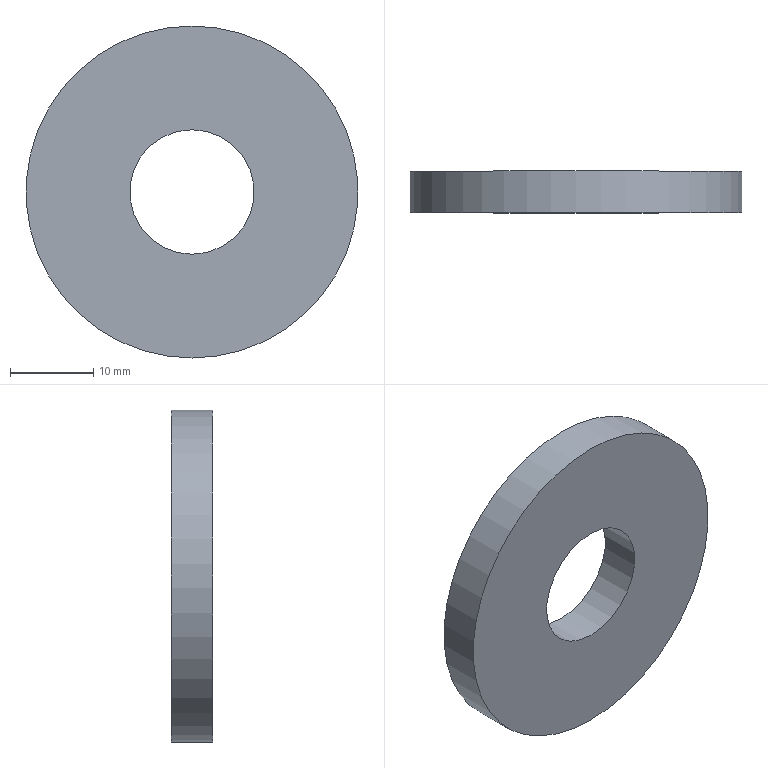Part | STEP file | HL4GZ-1.862.102 flat washer | 1 solid | 4 faces | box 40 x 5 x 40 mm | volume 5400 mm3 | plane 2 | cylinder 2 | commonest cylinder face diameters 15 x1 40 x1
STEP:
#1=CARTESIAN_POINT('',(0.,0.,0.));
#2=DIRECTION('',(0.,0.,1.));
#3=DIRECTION('',(1.,0.,0.));
#4=AXIS2_PLACEMENT_3D('',#1,#2,#3);
#5=CARTESIAN_POINT('',(1892.35,-249.5,-221.665));
#6=VERTEX_POINT('',#5);
#7=CARTESIAN_POINT('',(1885.318,-249.5,-219.057));
#8=DIRECTION('',(0.,1.,0.));
#9=DIRECTION('',(-0.9376,0.,0.3477));
#10=AXIS2_PLACEMENT_3D('',#7,#8,#9);
#11=CIRCLE('',#10,7.5);
#12=CARTESIAN_POINT('',(1885.318,-249.5,-219.057));
#13=DIRECTION('',(0.,-1.,0.));
#14=DIRECTION('',(-0.3477,0.,-0.9376));
#15=AXIS2_PLACEMENT_3D('',#12,#13,#14);
#16=PLANE('',#15);
#17=CARTESIAN_POINT('',(0.,-7.5));
#18=CARTESIAN_POINT('',(-12.99,-7.5));
#19=CARTESIAN_POINT('',(-6.495,3.75));
#20=CARTESIAN_POINT('',(0.,15.));
#21=CARTESIAN_POINT('',(6.495,3.75));
#22=CARTESIAN_POINT('',(12.99,-7.5));
#23=CARTESIAN_POINT('',(0.,-7.5));
#24=(BOUNDED_CURVE()B_SPLINE_CURVE(2,(#17,#18,#19,#20,#21,#22,#23),.UNSPECIFIED.,.T.,.F.)B_SPLINE_CURVE_WITH_KNOTS((1,2,2,2,2,1),(-2.094,0.,2.094,4.189,6.283,8.378),.UNSPECIFIED.)CURVE()GEOMETRIC_REPRESENTATION_ITEM()RATIONAL_B_SPLINE_CURVE((1.,0.5,1.,0.5,1.,0.5,1.))REPRESENTATION_ITEM(''));
#25=(GEOMETRIC_REPRESENTATION_CONTEXT(2)PARAMETRIC_REPRESENTATION_CONTEXT()REPRESENTATION_CONTEXT('',''));
#26=DEFINITIONAL_REPRESENTATION('',(#24),#25);
#27=PCURVE('',#16,#26);
#28=CARTESIAN_POINT('',(1885.318,-247.5,-219.057));
#29=DIRECTION('',(0.,1.,0.));
#30=DIRECTION('',(-0.9376,0.,0.3477));
#31=AXIS2_PLACEMENT_3D('',#28,#29,#30);
#32=CYLINDRICAL_SURFACE('',#31,7.5);
#33=CARTESIAN_POINT('',(0.,-2.));
#34=DIRECTION('',(1.,0.));
#35=VECTOR('',#34,1.);
#36=LINE('',#33,#35);
#37=(GEOMETRIC_REPRESENTATION_CONTEXT(2)PARAMETRIC_REPRESENTATION_CONTEXT()REPRESENTATION_CONTEXT('',''));
#38=DEFINITIONAL_REPRESENTATION('',(#36),#37);
#39=PCURVE('',#32,#38);
#40=SURFACE_CURVE('',#11,(#27,#39),.PCURVE_S1.);
#41=EDGE_CURVE('',#6,#6,#40,.T.);
#42=ORIENTED_EDGE('',*,*,#41,.T.);
#43=EDGE_LOOP('',(#42));
#44=FACE_BOUND('',#43,.T.);
#45=CARTESIAN_POINT('',(1885.318,-249.5,-239.057));
#46=VERTEX_POINT('',#45);
#47=CARTESIAN_POINT('',(1885.318,-249.5,-219.057));
#48=DIRECTION('',(0.,-1.,0.));
#49=DIRECTION('',(0.,0.,-1.));
#50=AXIS2_PLACEMENT_3D('',#47,#48,#49);
#51=CIRCLE('',#50,20.);
#52=CARTESIAN_POINT('',(0.,0.));
#53=DIRECTION('',(0.9376,0.3477));
#54=AXIS2_PLACEMENT_2D('',#52,#53);
#55=CIRCLE('',#54,20.);
#56=(GEOMETRIC_REPRESENTATION_CONTEXT(2)PARAMETRIC_REPRESENTATION_CONTEXT()REPRESENTATION_CONTEXT('',''));
#57=DEFINITIONAL_REPRESENTATION('',(#55),#56);
#58=PCURVE('',#16,#57);
#59=CARTESIAN_POINT('',(1885.318,-247.5,-219.057));
#60=DIRECTION('',(0.,1.,0.));
#61=DIRECTION('',(-0.9376,0.,0.3477));
#62=AXIS2_PLACEMENT_3D('',#59,#60,#61);
#63=CYLINDRICAL_SURFACE('',#62,20.);
#64=CARTESIAN_POINT('',(10.64,-2.));
#65=DIRECTION('',(-1.,0.));
#66=VECTOR('',#65,1.);
#67=LINE('',#64,#66);
#68=(GEOMETRIC_REPRESENTATION_CONTEXT(2)PARAMETRIC_REPRESENTATION_CONTEXT()REPRESENTATION_CONTEXT('',''));
#69=DEFINITIONAL_REPRESENTATION('',(#67),#68);
#70=PCURVE('',#63,#69);
#71=SURFACE_CURVE('',#51,(#58,#70),.PCURVE_S1.);
#72=EDGE_CURVE('',#46,#46,#71,.T.);
#73=ORIENTED_EDGE('',*,*,#72,.T.);
#74=EDGE_LOOP('',(#73));
#75=FACE_BOUND('',#74,.T.);
#76=ADVANCED_FACE('',(#44,#75),#16,.T.);
#77=CARTESIAN_POINT('',(1892.35,-244.5,-221.665));
#78=VERTEX_POINT('',#77);
#79=CARTESIAN_POINT('',(1885.318,-244.5,-219.057));
#80=DIRECTION('',(0.,-1.,0.));
#81=DIRECTION('',(-0.9376,0.,0.3477));
#82=AXIS2_PLACEMENT_3D('',#79,#80,#81);
#83=CIRCLE('',#82,7.5);
#84=CARTESIAN_POINT('',(1885.318,-244.5,-219.057));
#85=DIRECTION('',(0.,-1.,0.));
#86=DIRECTION('',(-0.3477,0.,-0.9376));
#87=AXIS2_PLACEMENT_3D('',#84,#85,#86);
#88=PLANE('',#87);
#89=CARTESIAN_POINT('',(0.,0.));
#90=DIRECTION('',(0.,-1.));
#91=AXIS2_PLACEMENT_2D('',#89,#90);
#92=CIRCLE('',#91,7.5);
#93=(GEOMETRIC_REPRESENTATION_CONTEXT(2)PARAMETRIC_REPRESENTATION_CONTEXT()REPRESENTATION_CONTEXT('',''));
#94=DEFINITIONAL_REPRESENTATION('',(#92),#93);
#95=PCURVE('',#88,#94);
#96=CARTESIAN_POINT('',(12.566,3.));
#97=DIRECTION('',(-1.,0.));
#98=VECTOR('',#97,1.);
#99=LINE('',#96,#98);
#100=(GEOMETRIC_REPRESENTATION_CONTEXT(2)PARAMETRIC_REPRESENTATION_CONTEXT()REPRESENTATION_CONTEXT('',''));
#101=DEFINITIONAL_REPRESENTATION('',(#99),#100);
#102=PCURVE('',#32,#101);
#103=SURFACE_CURVE('',#83,(#95,#102),.PCURVE_S1.);
#104=EDGE_CURVE('',#78,#78,#103,.T.);
#105=ORIENTED_EDGE('',*,*,#104,.T.);
#106=EDGE_LOOP('',(#105));
#107=FACE_BOUND('',#106,.T.);
#108=CARTESIAN_POINT('',(1885.318,-244.5,-239.057));
#109=VERTEX_POINT('',#108);
#110=CARTESIAN_POINT('',(1885.318,-244.5,-219.057));
#111=DIRECTION('',(0.,-1.,0.));
#112=DIRECTION('',(0.,0.,-1.));
#113=AXIS2_PLACEMENT_3D('',#110,#111,#112);
#114=CIRCLE('',#113,20.);
#115=CARTESIAN_POINT('',(0.,0.));
#116=DIRECTION('',(0.9376,0.3477));
#117=AXIS2_PLACEMENT_2D('',#115,#116);
#118=CIRCLE('',#117,20.);
#119=(GEOMETRIC_REPRESENTATION_CONTEXT(2)PARAMETRIC_REPRESENTATION_CONTEXT()REPRESENTATION_CONTEXT('',''));
#120=DEFINITIONAL_REPRESENTATION('',(#118),#119);
#121=PCURVE('',#88,#120);
#122=CARTESIAN_POINT('',(10.64,3.));
#123=DIRECTION('',(-1.,0.));
#124=VECTOR('',#123,1.);
#125=LINE('',#122,#124);
#126=(GEOMETRIC_REPRESENTATION_CONTEXT(2)PARAMETRIC_REPRESENTATION_CONTEXT()REPRESENTATION_CONTEXT('',''));
#127=DEFINITIONAL_REPRESENTATION('',(#125),#126);
#128=PCURVE('',#63,#127);
#129=SURFACE_CURVE('',#114,(#121,#128),.PCURVE_S1.);
#130=EDGE_CURVE('',#109,#109,#129,.T.);
#131=ORIENTED_EDGE('',*,*,#130,.F.);
#132=EDGE_LOOP('',(#131));
#133=FACE_BOUND('',#132,.T.);
#134=ADVANCED_FACE('',(#107,#133),#88,.F.);
#135=ORIENTED_EDGE('',*,*,#72,.F.);
#136=CARTESIAN_POINT('',(1885.318,-249.5,-239.057));
#137=CARTESIAN_POINT('',(1885.318,-244.5,-239.057));
#138=B_SPLINE_CURVE_WITH_KNOTS('',1,(#136,#137),.UNSPECIFIED.,.F.,.F.,(2,2),(-2.,3.),.PIECEWISE_BEZIER_KNOTS.);
#139=CARTESIAN_POINT('',(10.64,0.));
#140=DIRECTION('',(0.,1.));
#141=VECTOR('',#140,1.);
#142=LINE('',#139,#141);
#143=(GEOMETRIC_REPRESENTATION_CONTEXT(2)PARAMETRIC_REPRESENTATION_CONTEXT()REPRESENTATION_CONTEXT('',''));
#144=DEFINITIONAL_REPRESENTATION('',(#142),#143);
#145=PCURVE('',#63,#144);
#146=CARTESIAN_POINT('',(4.357,0.));
#147=DIRECTION('',(0.,1.));
#148=VECTOR('',#147,1.);
#149=LINE('',#146,#148);
#150=(GEOMETRIC_REPRESENTATION_CONTEXT(2)PARAMETRIC_REPRESENTATION_CONTEXT()REPRESENTATION_CONTEXT('',''));
#151=DEFINITIONAL_REPRESENTATION('',(#149),#150);
#152=PCURVE('',#63,#151);
#153=SEAM_CURVE('',#138,(#145,#152),.PCURVE_S1.);
#154=EDGE_CURVE('',#46,#109,#153,.T.);
#155=ORIENTED_EDGE('',*,*,#154,.T.);
#156=ORIENTED_EDGE('',*,*,#130,.T.);
#157=ORIENTED_EDGE('',*,*,#154,.F.);
#158=EDGE_LOOP('',(#135,#155,#156,#157));
#159=FACE_BOUND('',#158,.T.);
#160=ADVANCED_FACE('',(#159),#63,.T.);
#161=ORIENTED_EDGE('',*,*,#41,.T.);
#162=CARTESIAN_POINT('',(1892.35,-249.5,-221.665));
#163=CARTESIAN_POINT('',(1892.35,-244.5,-221.665));
#164=B_SPLINE_CURVE_WITH_KNOTS('',1,(#162,#163),.UNSPECIFIED.,.F.,.F.,(2,2),(-2.,3.),.PIECEWISE_BEZIER_KNOTS.);
#165=CARTESIAN_POINT('',(9.425,0.));
#166=DIRECTION('',(0.,1.));
#167=VECTOR('',#166,1.);
#168=LINE('',#165,#167);
#169=(GEOMETRIC_REPRESENTATION_CONTEXT(2)PARAMETRIC_REPRESENTATION_CONTEXT()REPRESENTATION_CONTEXT('',''));
#170=DEFINITIONAL_REPRESENTATION('',(#168),#169);
#171=PCURVE('',#32,#170);
#172=CARTESIAN_POINT('',(3.142,0.));
#173=DIRECTION('',(0.,1.));
#174=VECTOR('',#173,1.);
#175=LINE('',#172,#174);
#176=(GEOMETRIC_REPRESENTATION_CONTEXT(2)PARAMETRIC_REPRESENTATION_CONTEXT()REPRESENTATION_CONTEXT('',''));
#177=DEFINITIONAL_REPRESENTATION('',(#175),#176);
#178=PCURVE('',#32,#177);
#179=SEAM_CURVE('',#164,(#171,#178),.PCURVE_S1.);
#180=EDGE_CURVE('',#6,#78,#179,.T.);
#181=ORIENTED_EDGE('',*,*,#180,.T.);
#182=ORIENTED_EDGE('',*,*,#104,.T.);
#183=ORIENTED_EDGE('',*,*,#180,.F.);
#184=EDGE_LOOP('',(#161,#181,#182,#183));
#185=FACE_BOUND('',#184,.F.);
#186=ADVANCED_FACE('',(#185),#32,.F.);
#187=CLOSED_SHELL('',(#76,#134,#160,#186));
#188=MANIFOLD_SOLID_BREP('',#187);
#189=(LENGTH_UNIT()NAMED_UNIT(*)SI_UNIT(.MILLI.,.METRE.));
#190=UNCERTAINTY_MEASURE_WITH_UNIT(LENGTH_MEASURE(0.00001),#189,'','');
#191=(NAMED_UNIT(*)PLANE_ANGLE_UNIT()SI_UNIT($,.RADIAN.));
#192=(NAMED_UNIT(*)SI_UNIT($,.STERADIAN.)SOLID_ANGLE_UNIT());
#193=(GEOMETRIC_REPRESENTATION_CONTEXT(3)GLOBAL_UNCERTAINTY_ASSIGNED_CONTEXT((#190))GLOBAL_UNIT_ASSIGNED_CONTEXT((#189,#191,#192))REPRESENTATION_CONTEXT('',''));
#194=ADVANCED_BREP_SHAPE_REPRESENTATION('',(#4,#188),#193);